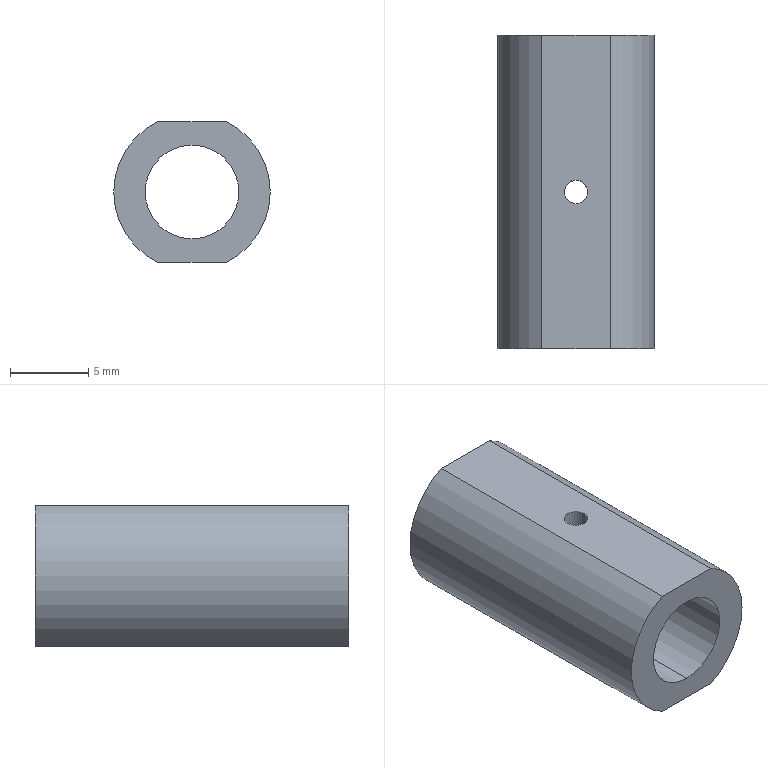Part | SolidWorks | features Extrusion 1, ICE 1 | 1 solid | 12 faces | box 10 x 20 x 9 mm | volume 941.197 mm3 | cylinder 8 | plane 4 | commonest cylinder face diameters 1.5 x4 6 x2 10 x2
STEP:
#1=CARTESIAN_POINT('',(0.,9.25,-3.));
#2=VERTEX_POINT('',#1);
#3=CARTESIAN_POINT('',(0.75,10.,-2.905));
#4=VERTEX_POINT('',#3);
#5=CARTESIAN_POINT('',(0.,9.25,-3.));
#6=CARTESIAN_POINT('',(0.09812,9.25,-3.));
#7=CARTESIAN_POINT('',(0.1972,9.27,-2.995));
#8=CARTESIAN_POINT('',(0.3779,9.345,-2.977));
#9=CARTESIAN_POINT('',(0.461,9.4,-2.965));
#10=CARTESIAN_POINT('',(0.6686,9.608,-2.928));
#11=CARTESIAN_POINT('',(0.75,9.802,-2.905));
#12=CARTESIAN_POINT('',(0.75,10.,-2.905));
#13=B_SPLINE_CURVE_WITH_KNOTS('',3,(#5,#6,#7,#8,#9,#10,#11,#12),.UNSPECIFIED.,.F.,.F.,(4,2,2,4),(0.002354,0.002648,0.002943,0.003531),.UNSPECIFIED.);
#14=EDGE_CURVE('',#2,#4,#13,.T.);
#15=ORIENTED_EDGE('',*,*,#14,.T.);
#16=CARTESIAN_POINT('',(0.75,10.,-4.5));
#17=VERTEX_POINT('',#16);
#18=CARTESIAN_POINT('',(0.75,10.,15.5));
#19=DIRECTION('',(0.,0.,-1.));
#20=VECTOR('',#19,1000.);
#21=LINE('',#18,#20);
#22=EDGE_CURVE('',#4,#17,#21,.T.);
#23=ORIENTED_EDGE('',*,*,#22,.T.);
#24=CARTESIAN_POINT('',(-0.75,10.,-4.5));
#25=VERTEX_POINT('',#24);
#26=CARTESIAN_POINT('',(0.,10.,-4.5));
#27=DIRECTION('',(0.,0.,-1.));
#28=DIRECTION('',(-1.,0.,0.));
#29=AXIS2_PLACEMENT_3D('',#26,#27,#28);
#30=CIRCLE('',#29,0.75);
#31=EDGE_CURVE('',#17,#25,#30,.T.);
#32=ORIENTED_EDGE('',*,*,#31,.T.);
#33=CARTESIAN_POINT('',(-0.75,10.,-2.905));
#34=VERTEX_POINT('',#33);
#35=CARTESIAN_POINT('',(-0.75,10.,15.5));
#36=DIRECTION('',(0.,0.,-1.));
#37=VECTOR('',#36,1000.);
#38=LINE('',#35,#37);
#39=EDGE_CURVE('',#34,#25,#38,.T.);
#40=ORIENTED_EDGE('',*,*,#39,.F.);
#41=CARTESIAN_POINT('',(-0.75,10.,-2.905));
#42=CARTESIAN_POINT('',(-0.75,9.902,-2.905));
#43=CARTESIAN_POINT('',(-0.7304,9.803,-2.91));
#44=CARTESIAN_POINT('',(-0.6548,9.621,-2.928));
#45=CARTESIAN_POINT('',(-0.5996,9.539,-2.94));
#46=CARTESIAN_POINT('',(-0.4606,9.4,-2.965));
#47=CARTESIAN_POINT('',(-0.378,9.345,-2.977));
#48=CARTESIAN_POINT('',(-0.1969,9.27,-2.995));
#49=CARTESIAN_POINT('',(-0.0981,9.25,-3.));
#50=CARTESIAN_POINT('',(0.,9.25,-3.));
#51=B_SPLINE_CURVE_WITH_KNOTS('',3,(#41,#42,#43,#44,#45,#46,#47,#48,#49,#50),.UNSPECIFIED.,.F.,.F.,(4,2,2,2,4),(0.001177,0.001472,0.001766,0.00206,0.002354),.UNSPECIFIED.);
#52=EDGE_CURVE('',#34,#2,#51,.T.);
#53=ORIENTED_EDGE('',*,*,#52,.T.);
#54=EDGE_LOOP('',(#15,#23,#32,#40,#53));
#55=FACE_OUTER_BOUND('',#54,.T.);
#56=CARTESIAN_POINT('',(0.,10.,15.5));
#57=DIRECTION('',(0.,0.,-1.));
#58=DIRECTION('',(-1.,0.,0.));
#59=AXIS2_PLACEMENT_3D('',#56,#57,#58);
#60=CYLINDRICAL_SURFACE('',#59,0.75);
#61=ADVANCED_FACE('',(#55),#60,.F.);
#62=CARTESIAN_POINT('',(-0.75,10.,4.5));
#63=VERTEX_POINT('',#62);
#64=CARTESIAN_POINT('',(0.75,10.,4.5));
#65=VERTEX_POINT('',#64);
#66=CARTESIAN_POINT('',(0.,10.,4.5));
#67=DIRECTION('',(0.,0.,1.));
#68=DIRECTION('',(1.,0.,0.));
#69=AXIS2_PLACEMENT_3D('',#66,#67,#68);
#70=CIRCLE('',#69,0.75);
#71=EDGE_CURVE('',#63,#65,#70,.T.);
#72=ORIENTED_EDGE('',*,*,#71,.T.);
#73=CARTESIAN_POINT('',(0.75,10.,2.905));
#74=VERTEX_POINT('',#73);
#75=CARTESIAN_POINT('',(0.75,10.,15.5));
#76=DIRECTION('',(0.,0.,-1.));
#77=VECTOR('',#76,1000.);
#78=LINE('',#75,#77);
#79=EDGE_CURVE('',#65,#74,#78,.T.);
#80=ORIENTED_EDGE('',*,*,#79,.T.);
#81=CARTESIAN_POINT('',(0.,9.25,3.));
#82=VERTEX_POINT('',#81);
#83=CARTESIAN_POINT('',(0.75,10.,2.905));
#84=CARTESIAN_POINT('',(0.75,9.902,2.905));
#85=CARTESIAN_POINT('',(0.7302,9.803,2.91));
#86=CARTESIAN_POINT('',(0.6552,9.622,2.928));
#87=CARTESIAN_POINT('',(0.5996,9.539,2.94));
#88=CARTESIAN_POINT('',(0.3922,9.331,2.978));
#89=CARTESIAN_POINT('',(0.1979,9.25,3.));
#90=CARTESIAN_POINT('',(0.,9.25,3.));
#91=B_SPLINE_CURVE_WITH_KNOTS('',3,(#83,#84,#85,#86,#87,#88,#89,#90),.UNSPECIFIED.,.F.,.F.,(4,2,2,4),(0.002354,0.002648,0.002943,0.003531),.UNSPECIFIED.);
#92=EDGE_CURVE('',#74,#82,#91,.T.);
#93=ORIENTED_EDGE('',*,*,#92,.T.);
#94=CARTESIAN_POINT('',(-0.75,10.,2.905));
#95=VERTEX_POINT('',#94);
#96=CARTESIAN_POINT('',(0.,9.25,3.));
#97=CARTESIAN_POINT('',(-0.1978,9.25,3.));
#98=CARTESIAN_POINT('',(-0.3925,9.332,2.978));
#99=CARTESIAN_POINT('',(-0.6678,9.607,2.928));
#100=CARTESIAN_POINT('',(-0.75,9.801,2.905));
#101=CARTESIAN_POINT('',(-0.75,10.,2.905));
#102=B_SPLINE_CURVE_WITH_KNOTS('',3,(#96,#97,#98,#99,#100,#101),.UNSPECIFIED.,.F.,.F.,(4,2,4),(0.003531,0.004119,0.004708),.UNSPECIFIED.);
#103=EDGE_CURVE('',#82,#95,#102,.T.);
#104=ORIENTED_EDGE('',*,*,#103,.T.);
#105=CARTESIAN_POINT('',(-0.75,10.,15.5));
#106=DIRECTION('',(0.,0.,-1.));
#107=VECTOR('',#106,1000.);
#108=LINE('',#105,#107);
#109=EDGE_CURVE('',#63,#95,#108,.T.);
#110=ORIENTED_EDGE('',*,*,#109,.F.);
#111=EDGE_LOOP('',(#72,#80,#93,#104,#110));
#112=FACE_OUTER_BOUND('',#111,.T.);
#113=CARTESIAN_POINT('',(0.,10.,15.5));
#114=DIRECTION('',(0.,0.,-1.));
#115=DIRECTION('',(-1.,0.,0.));
#116=AXIS2_PLACEMENT_3D('',#113,#114,#115);
#117=CYLINDRICAL_SURFACE('',#116,0.75);
#118=ADVANCED_FACE('',(#112),#117,.F.);
#119=CARTESIAN_POINT('',(0.,20.,-3.));
#120=VERTEX_POINT('',#119);
#121=CARTESIAN_POINT('',(0.,20.,3.));
#122=VERTEX_POINT('',#121);
#123=CARTESIAN_POINT('',(0.,20.,0.));
#124=DIRECTION('',(0.,1.,0.));
#125=DIRECTION('',(0.,0.,1.));
#126=AXIS2_PLACEMENT_3D('',#123,#124,#125);
#127=CIRCLE('',#126,3.);
#128=EDGE_CURVE('',#120,#122,#127,.T.);
#129=ORIENTED_EDGE('',*,*,#128,.T.);
#130=CARTESIAN_POINT('',(0.,10.75,3.));
#131=VERTEX_POINT('',#130);
#132=CARTESIAN_POINT('',(0.,20.,3.));
#133=DIRECTION('',(0.,-1.,0.));
#134=VECTOR('',#133,1000.);
#135=LINE('',#132,#134);
#136=EDGE_CURVE('',#122,#131,#135,.T.);
#137=ORIENTED_EDGE('',*,*,#136,.T.);
#138=CARTESIAN_POINT('',(-0.75,10.,2.905));
#139=CARTESIAN_POINT('',(-0.75,10.1,2.905));
#140=CARTESIAN_POINT('',(-0.7302,10.197,2.91));
#141=CARTESIAN_POINT('',(-0.6548,10.379,2.928));
#142=CARTESIAN_POINT('',(-0.599,10.462,2.94));
#143=CARTESIAN_POINT('',(-0.4612,10.599,2.965));
#144=CARTESIAN_POINT('',(-0.3778,10.655,2.978));
#145=CARTESIAN_POINT('',(-0.1973,10.73,2.995));
#146=CARTESIAN_POINT('',(-0.09831,10.75,3.));
#147=CARTESIAN_POINT('',(0.,10.75,3.));
#148=B_SPLINE_CURVE_WITH_KNOTS('',3,(#138,#139,#140,#141,#142,#143,#144,#145,#146,#147),.UNSPECIFIED.,.F.,.F.,(4,2,2,2,4),(0.,0.0002944,0.0005887,0.0008831,0.001177),.UNSPECIFIED.);
#149=EDGE_CURVE('',#95,#131,#148,.T.);
#150=ORIENTED_EDGE('',*,*,#149,.F.);
#151=ORIENTED_EDGE('',*,*,#103,.F.);
#152=CARTESIAN_POINT('',(0.,0.,3.));
#153=VERTEX_POINT('',#152);
#154=CARTESIAN_POINT('',(0.,20.,3.));
#155=DIRECTION('',(0.,-1.,0.));
#156=VECTOR('',#155,1000.);
#157=LINE('',#154,#156);
#158=EDGE_CURVE('',#82,#153,#157,.T.);
#159=ORIENTED_EDGE('',*,*,#158,.T.);
#160=CARTESIAN_POINT('',(0.,0.,-3.));
#161=VERTEX_POINT('',#160);
#162=CARTESIAN_POINT('',(0.,0.,0.));
#163=DIRECTION('',(0.,1.,0.));
#164=DIRECTION('',(0.,0.,1.));
#165=AXIS2_PLACEMENT_3D('',#162,#163,#164);
#166=CIRCLE('',#165,3.);
#167=EDGE_CURVE('',#161,#153,#166,.T.);
#168=ORIENTED_EDGE('',*,*,#167,.F.);
#169=CARTESIAN_POINT('',(0.,20.,-3.));
#170=DIRECTION('',(0.,-1.,0.));
#171=VECTOR('',#170,1000.);
#172=LINE('',#169,#171);
#173=EDGE_CURVE('',#2,#161,#172,.T.);
#174=ORIENTED_EDGE('',*,*,#173,.F.);
#175=ORIENTED_EDGE('',*,*,#52,.F.);
#176=CARTESIAN_POINT('',(0.,10.75,-3.));
#177=VERTEX_POINT('',#176);
#178=CARTESIAN_POINT('',(0.,10.75,-3.));
#179=CARTESIAN_POINT('',(-0.09956,10.75,-3.));
#180=CARTESIAN_POINT('',(-0.1972,10.73,-2.995));
#181=CARTESIAN_POINT('',(-0.3788,10.655,-2.977));
#182=CARTESIAN_POINT('',(-0.4617,10.599,-2.965));
#183=CARTESIAN_POINT('',(-0.5995,10.461,-2.94));
#184=CARTESIAN_POINT('',(-0.6553,10.378,-2.928));
#185=CARTESIAN_POINT('',(-0.7301,10.197,-2.91));
#186=CARTESIAN_POINT('',(-0.75,10.098,-2.905));
#187=CARTESIAN_POINT('',(-0.75,10.,-2.905));
#188=B_SPLINE_CURVE_WITH_KNOTS('',3,(#178,#179,#180,#181,#182,#183,#184,#185,#186,#187),.UNSPECIFIED.,.F.,.F.,(4,2,2,2,4),(0.,0.0002944,0.0005887,0.0008831,0.001177),.UNSPECIFIED.);
#189=EDGE_CURVE('',#177,#34,#188,.T.);
#190=ORIENTED_EDGE('',*,*,#189,.F.);
#191=CARTESIAN_POINT('',(0.,20.,-3.));
#192=DIRECTION('',(0.,-1.,0.));
#193=VECTOR('',#192,1000.);
#194=LINE('',#191,#193);
#195=EDGE_CURVE('',#120,#177,#194,.T.);
#196=ORIENTED_EDGE('',*,*,#195,.F.);
#197=EDGE_LOOP('',(#129,#137,#150,#151,#159,#168,#174,#175,#190,#196));
#198=FACE_OUTER_BOUND('',#197,.T.);
#199=CARTESIAN_POINT('',(0.,20.,0.));
#200=DIRECTION('',(0.,-1.,0.));
#201=DIRECTION('',(0.,0.,-1.));
#202=AXIS2_PLACEMENT_3D('',#199,#200,#201);
#203=CYLINDRICAL_SURFACE('',#202,3.);
#204=ADVANCED_FACE('',(#198),#203,.F.);
#205=ORIENTED_EDGE('',*,*,#71,.F.);
#206=CARTESIAN_POINT('',(0.,10.,4.5));
#207=DIRECTION('',(0.,0.,1.));
#208=DIRECTION('',(1.,0.,0.));
#209=AXIS2_PLACEMENT_3D('',#206,#207,#208);
#210=CIRCLE('',#209,0.75);
#211=EDGE_CURVE('',#65,#63,#210,.T.);
#212=ORIENTED_EDGE('',*,*,#211,.F.);
#213=EDGE_LOOP('',(#205,#212));
#214=FACE_BOUND('',#213,.T.);
#215=CARTESIAN_POINT('',(2.179,0.,4.5));
#216=VERTEX_POINT('',#215);
#217=CARTESIAN_POINT('',(-2.179,0.,4.5));
#218=VERTEX_POINT('',#217);
#219=CARTESIAN_POINT('',(0.,0.,4.5));
#220=DIRECTION('',(-1.,0.,0.));
#221=VECTOR('',#220,1000.);
#222=LINE('',#219,#221);
#223=EDGE_CURVE('',#216,#218,#222,.T.);
#224=ORIENTED_EDGE('',*,*,#223,.F.);
#225=CARTESIAN_POINT('',(2.179,20.,4.5));
#226=VERTEX_POINT('',#225);
#227=CARTESIAN_POINT('',(2.179,20.,4.5));
#228=DIRECTION('',(0.,-1.,0.));
#229=VECTOR('',#228,1000.);
#230=LINE('',#227,#229);
#231=EDGE_CURVE('',#226,#216,#230,.T.);
#232=ORIENTED_EDGE('',*,*,#231,.F.);
#233=CARTESIAN_POINT('',(-2.179,20.,4.5));
#234=VERTEX_POINT('',#233);
#235=CARTESIAN_POINT('',(0.,20.,4.5));
#236=DIRECTION('',(-1.,0.,0.));
#237=VECTOR('',#236,1000.);
#238=LINE('',#235,#237);
#239=EDGE_CURVE('',#226,#234,#238,.T.);
#240=ORIENTED_EDGE('',*,*,#239,.T.);
#241=CARTESIAN_POINT('',(-2.179,20.,4.5));
#242=DIRECTION('',(0.,-1.,0.));
#243=VECTOR('',#242,1000.);
#244=LINE('',#241,#243);
#245=EDGE_CURVE('',#234,#218,#244,.T.);
#246=ORIENTED_EDGE('',*,*,#245,.T.);
#247=EDGE_LOOP('',(#224,#232,#240,#246));
#248=FACE_OUTER_BOUND('',#247,.T.);
#249=CARTESIAN_POINT('',(0.,20.,4.5));
#250=DIRECTION('',(0.,0.,1.));
#251=DIRECTION('',(1.,0.,0.));
#252=AXIS2_PLACEMENT_3D('',#249,#250,#251);
#253=PLANE('',#252);
#254=ADVANCED_FACE('',(#214,#248),#253,.T.);
#255=CARTESIAN_POINT('',(2.179,0.,-4.5));
#256=VERTEX_POINT('',#255);
#257=CARTESIAN_POINT('',(0.,0.,0.));
#258=DIRECTION('',(0.,1.,0.));
#259=DIRECTION('',(0.,0.,1.));
#260=AXIS2_PLACEMENT_3D('',#257,#258,#259);
#261=CIRCLE('',#260,5.);
#262=EDGE_CURVE('',#216,#256,#261,.T.);
#263=ORIENTED_EDGE('',*,*,#262,.T.);
#264=CARTESIAN_POINT('',(2.179,20.,-4.5));
#265=VERTEX_POINT('',#264);
#266=CARTESIAN_POINT('',(2.179,20.,-4.5));
#267=DIRECTION('',(0.,-1.,0.));
#268=VECTOR('',#267,1000.);
#269=LINE('',#266,#268);
#270=EDGE_CURVE('',#265,#256,#269,.T.);
#271=ORIENTED_EDGE('',*,*,#270,.F.);
#272=CARTESIAN_POINT('',(0.,20.,0.));
#273=DIRECTION('',(0.,1.,0.));
#274=DIRECTION('',(0.,0.,1.));
#275=AXIS2_PLACEMENT_3D('',#272,#273,#274);
#276=CIRCLE('',#275,5.);
#277=EDGE_CURVE('',#226,#265,#276,.T.);
#278=ORIENTED_EDGE('',*,*,#277,.F.);
#279=ORIENTED_EDGE('',*,*,#231,.T.);
#280=EDGE_LOOP('',(#263,#271,#278,#279));
#281=FACE_OUTER_BOUND('',#280,.T.);
#282=CARTESIAN_POINT('',(0.,20.,0.));
#283=DIRECTION('',(0.,-1.,0.));
#284=DIRECTION('',(0.,0.,-1.));
#285=AXIS2_PLACEMENT_3D('',#282,#283,#284);
#286=CYLINDRICAL_SURFACE('',#285,5.);
#287=ADVANCED_FACE('',(#281),#286,.T.);
#288=CARTESIAN_POINT('',(0.,10.,-4.5));
#289=DIRECTION('',(0.,0.,-1.));
#290=DIRECTION('',(-1.,0.,0.));
#291=AXIS2_PLACEMENT_3D('',#288,#289,#290);
#292=CIRCLE('',#291,0.75);
#293=EDGE_CURVE('',#25,#17,#292,.T.);
#294=ORIENTED_EDGE('',*,*,#293,.F.);
#295=ORIENTED_EDGE('',*,*,#31,.F.);
#296=EDGE_LOOP('',(#294,#295));
#297=FACE_BOUND('',#296,.T.);
#298=CARTESIAN_POINT('',(-2.179,0.,-4.5));
#299=VERTEX_POINT('',#298);
#300=CARTESIAN_POINT('',(0.,0.,-4.5));
#301=DIRECTION('',(-1.,0.,0.));
#302=VECTOR('',#301,1000.);
#303=LINE('',#300,#302);
#304=EDGE_CURVE('',#256,#299,#303,.T.);
#305=ORIENTED_EDGE('',*,*,#304,.T.);
#306=CARTESIAN_POINT('',(-2.179,20.,-4.5));
#307=VERTEX_POINT('',#306);
#308=CARTESIAN_POINT('',(-2.179,20.,-4.5));
#309=DIRECTION('',(0.,-1.,0.));
#310=VECTOR('',#309,1000.);
#311=LINE('',#308,#310);
#312=EDGE_CURVE('',#307,#299,#311,.T.);
#313=ORIENTED_EDGE('',*,*,#312,.F.);
#314=CARTESIAN_POINT('',(0.,20.,-4.5));
#315=DIRECTION('',(-1.,0.,0.));
#316=VECTOR('',#315,1000.);
#317=LINE('',#314,#316);
#318=EDGE_CURVE('',#265,#307,#317,.T.);
#319=ORIENTED_EDGE('',*,*,#318,.F.);
#320=ORIENTED_EDGE('',*,*,#270,.T.);
#321=EDGE_LOOP('',(#305,#313,#319,#320));
#322=FACE_OUTER_BOUND('',#321,.T.);
#323=CARTESIAN_POINT('',(0.,20.,-4.5));
#324=DIRECTION('',(0.,0.,1.));
#325=DIRECTION('',(1.,0.,0.));
#326=AXIS2_PLACEMENT_3D('',#323,#324,#325);
#327=PLANE('',#326);
#328=ADVANCED_FACE('',(#297,#322),#327,.F.);
#329=ORIENTED_EDGE('',*,*,#136,.F.);
#330=CARTESIAN_POINT('',(0.,20.,0.));
#331=DIRECTION('',(0.,1.,0.));
#332=DIRECTION('',(0.,0.,1.));
#333=AXIS2_PLACEMENT_3D('',#330,#331,#332);
#334=CIRCLE('',#333,3.);
#335=EDGE_CURVE('',#122,#120,#334,.T.);
#336=ORIENTED_EDGE('',*,*,#335,.T.);
#337=ORIENTED_EDGE('',*,*,#195,.T.);
#338=CARTESIAN_POINT('',(0.75,10.,-2.905));
#339=CARTESIAN_POINT('',(0.75,10.198,-2.905));
#340=CARTESIAN_POINT('',(0.6681,10.392,-2.928));
#341=CARTESIAN_POINT('',(0.393,10.668,-2.977));
#342=CARTESIAN_POINT('',(0.199,10.75,-3.));
#343=CARTESIAN_POINT('',(0.,10.75,-3.));
#344=B_SPLINE_CURVE_WITH_KNOTS('',3,(#338,#339,#340,#341,#342,#343),.UNSPECIFIED.,.F.,.F.,(4,2,4),(0.003531,0.00412,0.004708),.UNSPECIFIED.);
#345=EDGE_CURVE('',#4,#177,#344,.T.);
#346=ORIENTED_EDGE('',*,*,#345,.F.);
#347=ORIENTED_EDGE('',*,*,#14,.F.);
#348=ORIENTED_EDGE('',*,*,#173,.T.);
#349=CARTESIAN_POINT('',(0.,0.,0.));
#350=DIRECTION('',(0.,1.,0.));
#351=DIRECTION('',(0.,0.,1.));
#352=AXIS2_PLACEMENT_3D('',#349,#350,#351);
#353=CIRCLE('',#352,3.);
#354=EDGE_CURVE('',#153,#161,#353,.T.);
#355=ORIENTED_EDGE('',*,*,#354,.F.);
#356=ORIENTED_EDGE('',*,*,#158,.F.);
#357=ORIENTED_EDGE('',*,*,#92,.F.);
#358=CARTESIAN_POINT('',(0.,10.75,3.));
#359=CARTESIAN_POINT('',(0.09826,10.75,3.));
#360=CARTESIAN_POINT('',(0.1967,10.73,2.995));
#361=CARTESIAN_POINT('',(0.3788,10.655,2.977));
#362=CARTESIAN_POINT('',(0.4612,10.6,2.965));
#363=CARTESIAN_POINT('',(0.6,10.461,2.94));
#364=CARTESIAN_POINT('',(0.6552,10.378,2.928));
#365=CARTESIAN_POINT('',(0.7303,10.197,2.91));
#366=CARTESIAN_POINT('',(0.75,10.098,2.905));
#367=CARTESIAN_POINT('',(0.75,10.,2.905));
#368=B_SPLINE_CURVE_WITH_KNOTS('',3,(#358,#359,#360,#361,#362,#363,#364,#365,#366,#367),.UNSPECIFIED.,.F.,.F.,(4,2,2,2,4),(0.001177,0.001472,0.001766,0.00206,0.002354),.UNSPECIFIED.);
#369=EDGE_CURVE('',#131,#74,#368,.T.);
#370=ORIENTED_EDGE('',*,*,#369,.F.);
#371=EDGE_LOOP('',(#329,#336,#337,#346,#347,#348,#355,#356,#357,#370));
#372=FACE_OUTER_BOUND('',#371,.T.);
#373=CARTESIAN_POINT('',(0.,20.,0.));
#374=DIRECTION('',(0.,-1.,0.));
#375=DIRECTION('',(0.,0.,-1.));
#376=AXIS2_PLACEMENT_3D('',#373,#374,#375);
#377=CYLINDRICAL_SURFACE('',#376,3.);
#378=ADVANCED_FACE('',(#372),#377,.F.);
#379=CARTESIAN_POINT('',(0.,0.,0.));
#380=DIRECTION('',(0.,1.,0.));
#381=DIRECTION('',(0.,0.,1.));
#382=AXIS2_PLACEMENT_3D('',#379,#380,#381);
#383=CIRCLE('',#382,5.);
#384=EDGE_CURVE('',#299,#218,#383,.T.);
#385=ORIENTED_EDGE('',*,*,#384,.T.);
#386=ORIENTED_EDGE('',*,*,#245,.F.);
#387=CARTESIAN_POINT('',(0.,20.,0.));
#388=DIRECTION('',(0.,1.,0.));
#389=DIRECTION('',(0.,0.,1.));
#390=AXIS2_PLACEMENT_3D('',#387,#388,#389);
#391=CIRCLE('',#390,5.);
#392=EDGE_CURVE('',#307,#234,#391,.T.);
#393=ORIENTED_EDGE('',*,*,#392,.F.);
#394=ORIENTED_EDGE('',*,*,#312,.T.);
#395=EDGE_LOOP('',(#385,#386,#393,#394));
#396=FACE_OUTER_BOUND('',#395,.T.);
#397=CARTESIAN_POINT('',(0.,20.,0.));
#398=DIRECTION('',(0.,-1.,0.));
#399=DIRECTION('',(0.,0.,-1.));
#400=AXIS2_PLACEMENT_3D('',#397,#398,#399);
#401=CYLINDRICAL_SURFACE('',#400,5.);
#402=ADVANCED_FACE('',(#396),#401,.T.);
#403=ORIENTED_EDGE('',*,*,#128,.F.);
#404=ORIENTED_EDGE('',*,*,#335,.F.);
#405=EDGE_LOOP('',(#403,#404));
#406=FACE_BOUND('',#405,.T.);
#407=ORIENTED_EDGE('',*,*,#239,.F.);
#408=ORIENTED_EDGE('',*,*,#277,.T.);
#409=ORIENTED_EDGE('',*,*,#318,.T.);
#410=ORIENTED_EDGE('',*,*,#392,.T.);
#411=EDGE_LOOP('',(#407,#408,#409,#410));
#412=FACE_OUTER_BOUND('',#411,.T.);
#413=CARTESIAN_POINT('',(0.,20.,0.));
#414=DIRECTION('',(0.,1.,0.));
#415=DIRECTION('',(0.,0.,1.));
#416=AXIS2_PLACEMENT_3D('',#413,#414,#415);
#417=PLANE('',#416);
#418=ADVANCED_FACE('',(#406,#412),#417,.T.);
#419=ORIENTED_EDGE('',*,*,#167,.T.);
#420=ORIENTED_EDGE('',*,*,#354,.T.);
#421=EDGE_LOOP('',(#419,#420));
#422=FACE_BOUND('',#421,.T.);
#423=ORIENTED_EDGE('',*,*,#223,.T.);
#424=ORIENTED_EDGE('',*,*,#384,.F.);
#425=ORIENTED_EDGE('',*,*,#304,.F.);
#426=ORIENTED_EDGE('',*,*,#262,.F.);
#427=EDGE_LOOP('',(#423,#424,#425,#426));
#428=FACE_OUTER_BOUND('',#427,.T.);
#429=CARTESIAN_POINT('',(0.,0.,0.));
#430=DIRECTION('',(0.,1.,0.));
#431=DIRECTION('',(0.,0.,1.));
#432=AXIS2_PLACEMENT_3D('',#429,#430,#431);
#433=PLANE('',#432);
#434=ADVANCED_FACE('',(#422,#428),#433,.F.);
#435=ORIENTED_EDGE('',*,*,#79,.F.);
#436=ORIENTED_EDGE('',*,*,#211,.T.);
#437=ORIENTED_EDGE('',*,*,#109,.T.);
#438=ORIENTED_EDGE('',*,*,#149,.T.);
#439=ORIENTED_EDGE('',*,*,#369,.T.);
#440=EDGE_LOOP('',(#435,#436,#437,#438,#439));
#441=FACE_OUTER_BOUND('',#440,.T.);
#442=CARTESIAN_POINT('',(0.,10.,15.5));
#443=DIRECTION('',(0.,0.,-1.));
#444=DIRECTION('',(-1.,0.,0.));
#445=AXIS2_PLACEMENT_3D('',#442,#443,#444);
#446=CYLINDRICAL_SURFACE('',#445,0.75);
#447=ADVANCED_FACE('',(#441),#446,.F.);
#448=ORIENTED_EDGE('',*,*,#22,.F.);
#449=ORIENTED_EDGE('',*,*,#345,.T.);
#450=ORIENTED_EDGE('',*,*,#189,.T.);
#451=ORIENTED_EDGE('',*,*,#39,.T.);
#452=ORIENTED_EDGE('',*,*,#293,.T.);
#453=EDGE_LOOP('',(#448,#449,#450,#451,#452));
#454=FACE_OUTER_BOUND('',#453,.T.);
#455=CARTESIAN_POINT('',(0.,10.,15.5));
#456=DIRECTION('',(0.,0.,-1.));
#457=DIRECTION('',(-1.,0.,0.));
#458=AXIS2_PLACEMENT_3D('',#455,#456,#457);
#459=CYLINDRICAL_SURFACE('',#458,0.75);
#460=ADVANCED_FACE('',(#454),#459,.F.);
#461=CLOSED_SHELL('',(#61,#118,#204,#254,#287,#328,#378,#402,#418,#434,#447,#460));
#462=MANIFOLD_SOLID_BREP('',#461);
#463=CARTESIAN_POINT('',(0.,0.,0.));
#464=DIRECTION('',(0.,0.,1.));
#465=DIRECTION('',(1.,0.,0.));
#466=AXIS2_PLACEMENT_3D('',#463,#464,#465);
#467=(LENGTH_UNIT()NAMED_UNIT(*)SI_UNIT(.MILLI.,.METRE.));
#468=UNCERTAINTY_MEASURE_WITH_UNIT(LENGTH_MEASURE(0.00001),#467,'','');
#469=(NAMED_UNIT(*)PLANE_ANGLE_UNIT()SI_UNIT($,.RADIAN.));
#470=(NAMED_UNIT(*)SI_UNIT($,.STERADIAN.)SOLID_ANGLE_UNIT());
#471=(GEOMETRIC_REPRESENTATION_CONTEXT(3)GLOBAL_UNCERTAINTY_ASSIGNED_CONTEXT((#468))GLOBAL_UNIT_ASSIGNED_CONTEXT((#467,#469,#470))REPRESENTATION_CONTEXT('',''));
#472=ADVANCED_BREP_SHAPE_REPRESENTATION('',(#462,#466),#471);